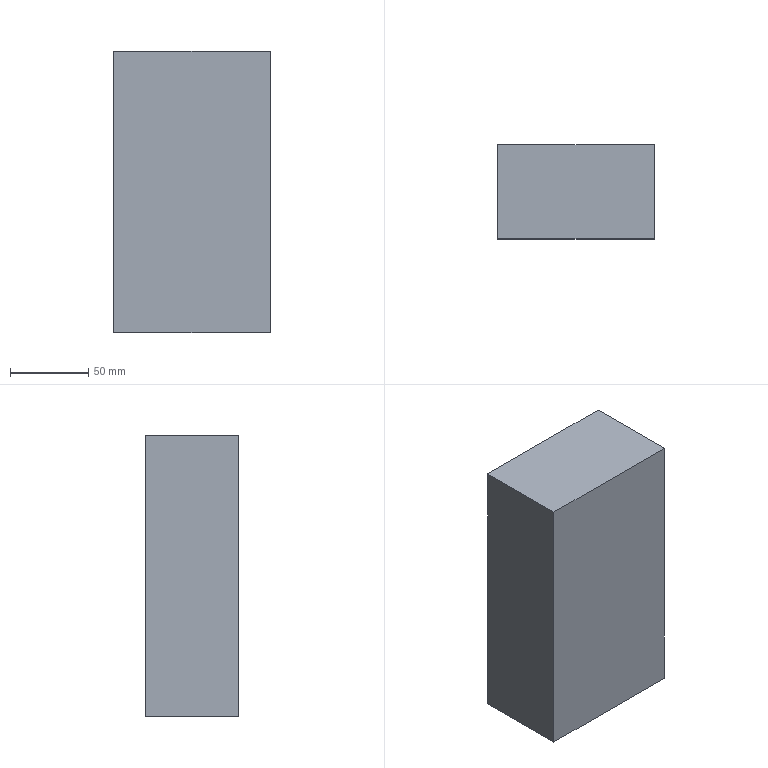Part | NX | features 28 2 | 1 solid | 10 faces | box 100 x 60 x 180 mm | volume 1074073 mm3 | plane 6 | cylinder 2 | cone 2 | commonest cylinder face diameters 10.3 x2
STEP:
#1=CARTESIAN_POINT('',(2254.85,742.5,-113.));
#2=VERTEX_POINT('',#1);
#3=CARTESIAN_POINT('',(2260.,742.5,-113.));
#4=DIRECTION('',(0.,0.,-1.));
#5=DIRECTION('',(-1.,0.,0.));
#6=AXIS2_PLACEMENT_3D('',#3,#4,#5);
#7=CIRCLE('',#6,5.15);
#8=EDGE_CURVE('',#2,#2,#7,.T.);
#9=ORIENTED_EDGE('',*,*,#8,.F.);
#10=EDGE_LOOP('',(#9));
#11=FACE_BOUND('',#10,.T.);
#12=CARTESIAN_POINT('',(2240.,712.5,-113.));
#13=VERTEX_POINT('',#12);
#14=CARTESIAN_POINT('',(2240.,772.5,-113.));
#15=VERTEX_POINT('',#14);
#16=CARTESIAN_POINT('',(2240.,387.5,-113.));
#17=DIRECTION('',(0.,1.,0.));
#18=VECTOR('',#17,1000.);
#19=LINE('',#16,#18);
#20=EDGE_CURVE('',#13,#15,#19,.T.);
#21=ORIENTED_EDGE('',*,*,#20,.T.);
#22=CARTESIAN_POINT('',(2340.,772.5,-113.));
#23=VERTEX_POINT('',#22);
#24=CARTESIAN_POINT('',(3179.121,772.5,-113.));
#25=DIRECTION('',(1.,0.,0.));
#26=VECTOR('',#25,1000.);
#27=LINE('',#24,#26);
#28=EDGE_CURVE('',#15,#23,#27,.T.);
#29=ORIENTED_EDGE('',*,*,#28,.T.);
#30=CARTESIAN_POINT('',(2340.,712.5,-113.));
#31=VERTEX_POINT('',#30);
#32=CARTESIAN_POINT('',(2340.,772.5,-113.));
#33=DIRECTION('',(0.,1.,0.));
#34=VECTOR('',#33,1000.);
#35=LINE('',#32,#34);
#36=EDGE_CURVE('',#31,#23,#35,.T.);
#37=ORIENTED_EDGE('',*,*,#36,.F.);
#38=CARTESIAN_POINT('',(3179.121,712.5,-113.));
#39=DIRECTION('',(-1.,0.,0.));
#40=VECTOR('',#39,1000.);
#41=LINE('',#38,#40);
#42=EDGE_CURVE('',#31,#13,#41,.T.);
#43=ORIENTED_EDGE('',*,*,#42,.T.);
#44=EDGE_LOOP('',(#21,#29,#37,#43));
#45=FACE_BOUND('',#44,.T.);
#46=CARTESIAN_POINT('',(2314.85,742.5,-113.));
#47=VERTEX_POINT('',#46);
#48=CARTESIAN_POINT('',(2320.,742.5,-113.));
#49=DIRECTION('',(0.,0.,-1.));
#50=DIRECTION('',(-1.,0.,0.));
#51=AXIS2_PLACEMENT_3D('',#48,#49,#50);
#52=CIRCLE('',#51,5.15);
#53=EDGE_CURVE('',#47,#47,#52,.T.);
#54=ORIENTED_EDGE('',*,*,#53,.F.);
#55=EDGE_LOOP('',(#54));
#56=FACE_BOUND('',#55,.T.);
#57=CARTESIAN_POINT('',(3179.121,387.5,-113.));
#58=DIRECTION('',(0.,0.,-1.));
#59=DIRECTION('',(1.,0.,0.));
#60=AXIS2_PLACEMENT_3D('',#57,#58,#59);
#61=PLANE('',#60);
#62=ADVANCED_FACE('',(#11,#45,#56),#61,.T.);
#63=CARTESIAN_POINT('',(2340.,712.5,67.));
#64=VERTEX_POINT('',#63);
#65=CARTESIAN_POINT('',(2240.,712.5,67.));
#66=VERTEX_POINT('',#65);
#67=CARTESIAN_POINT('',(4085.,712.5,67.));
#68=DIRECTION('',(-1.,0.,0.));
#69=VECTOR('',#68,1000.);
#70=LINE('',#67,#69);
#71=EDGE_CURVE('',#64,#66,#70,.T.);
#72=ORIENTED_EDGE('',*,*,#71,.F.);
#73=CARTESIAN_POINT('',(2340.,772.5,67.));
#74=VERTEX_POINT('',#73);
#75=CARTESIAN_POINT('',(2340.,572.5,67.));
#76=DIRECTION('',(0.,-1.,0.));
#77=VECTOR('',#76,1000.);
#78=LINE('',#75,#77);
#79=EDGE_CURVE('',#74,#64,#78,.T.);
#80=ORIENTED_EDGE('',*,*,#79,.F.);
#81=CARTESIAN_POINT('',(2240.,772.5,67.));
#82=VERTEX_POINT('',#81);
#83=CARTESIAN_POINT('',(4085.,772.5,67.));
#84=DIRECTION('',(1.,0.,0.));
#85=VECTOR('',#84,1000.);
#86=LINE('',#83,#85);
#87=EDGE_CURVE('',#82,#74,#86,.T.);
#88=ORIENTED_EDGE('',*,*,#87,.F.);
#89=CARTESIAN_POINT('',(2240.,572.5,67.));
#90=DIRECTION('',(0.,1.,0.));
#91=VECTOR('',#90,1000.);
#92=LINE('',#89,#91);
#93=EDGE_CURVE('',#66,#82,#92,.T.);
#94=ORIENTED_EDGE('',*,*,#93,.F.);
#95=EDGE_LOOP('',(#72,#80,#88,#94));
#96=FACE_BOUND('',#95,.T.);
#97=CARTESIAN_POINT('',(4085.,572.5,67.));
#98=DIRECTION('',(0.,0.,1.));
#99=DIRECTION('',(0.,1.,0.));
#100=AXIS2_PLACEMENT_3D('',#97,#98,#99);
#101=PLANE('',#100);
#102=ADVANCED_FACE('',(#96),#101,.T.);
#103=CARTESIAN_POINT('',(2340.,712.5,-113.));
#104=DIRECTION('',(0.,0.,-1.));
#105=VECTOR('',#104,1000.);
#106=LINE('',#103,#105);
#107=EDGE_CURVE('',#64,#31,#106,.T.);
#108=ORIENTED_EDGE('',*,*,#107,.T.);
#109=ORIENTED_EDGE('',*,*,#36,.T.);
#110=CARTESIAN_POINT('',(2340.,772.5,-113.));
#111=DIRECTION('',(0.,0.,1.));
#112=VECTOR('',#111,1000.);
#113=LINE('',#110,#112);
#114=EDGE_CURVE('',#23,#74,#113,.T.);
#115=ORIENTED_EDGE('',*,*,#114,.T.);
#116=ORIENTED_EDGE('',*,*,#79,.T.);
#117=EDGE_LOOP('',(#108,#109,#115,#116));
#118=FACE_BOUND('',#117,.T.);
#119=CARTESIAN_POINT('',(2340.,772.5,-113.));
#120=DIRECTION('',(1.,0.,0.));
#121=DIRECTION('',(0.,0.,1.));
#122=AXIS2_PLACEMENT_3D('',#119,#120,#121);
#123=PLANE('',#122);
#124=ADVANCED_FACE('',(#118),#123,.T.);
#125=ORIENTED_EDGE('',*,*,#114,.F.);
#126=ORIENTED_EDGE('',*,*,#28,.F.);
#127=CARTESIAN_POINT('',(2240.,772.5,-113.));
#128=DIRECTION('',(0.,0.,-1.));
#129=VECTOR('',#128,1000.);
#130=LINE('',#127,#129);
#131=EDGE_CURVE('',#82,#15,#130,.T.);
#132=ORIENTED_EDGE('',*,*,#131,.F.);
#133=ORIENTED_EDGE('',*,*,#87,.T.);
#134=EDGE_LOOP('',(#125,#126,#132,#133));
#135=FACE_BOUND('',#134,.T.);
#136=CARTESIAN_POINT('',(2270.,772.5,-113.));
#137=DIRECTION('',(0.,1.,0.));
#138=DIRECTION('',(0.,0.,1.));
#139=AXIS2_PLACEMENT_3D('',#136,#137,#138);
#140=PLANE('',#139);
#141=ADVANCED_FACE('',(#135),#140,.T.);
#142=ORIENTED_EDGE('',*,*,#131,.T.);
#143=ORIENTED_EDGE('',*,*,#20,.F.);
#144=CARTESIAN_POINT('',(2240.,712.5,-113.));
#145=DIRECTION('',(0.,0.,1.));
#146=VECTOR('',#145,1000.);
#147=LINE('',#144,#146);
#148=EDGE_CURVE('',#13,#66,#147,.T.);
#149=ORIENTED_EDGE('',*,*,#148,.T.);
#150=ORIENTED_EDGE('',*,*,#93,.T.);
#151=EDGE_LOOP('',(#142,#143,#149,#150));
#152=FACE_BOUND('',#151,.T.);
#153=CARTESIAN_POINT('',(2240.,772.5,-113.));
#154=DIRECTION('',(-1.,0.,0.));
#155=DIRECTION('',(0.,0.,-1.));
#156=AXIS2_PLACEMENT_3D('',#153,#154,#155);
#157=PLANE('',#156);
#158=ADVANCED_FACE('',(#152),#157,.T.);
#159=ORIENTED_EDGE('',*,*,#148,.F.);
#160=ORIENTED_EDGE('',*,*,#42,.F.);
#161=ORIENTED_EDGE('',*,*,#107,.F.);
#162=ORIENTED_EDGE('',*,*,#71,.T.);
#163=EDGE_LOOP('',(#159,#160,#161,#162));
#164=FACE_BOUND('',#163,.T.);
#165=CARTESIAN_POINT('',(2270.,712.5,-113.));
#166=DIRECTION('',(0.,-1.,0.));
#167=DIRECTION('',(0.,0.,-1.));
#168=AXIS2_PLACEMENT_3D('',#165,#166,#167);
#169=PLANE('',#168);
#170=ADVANCED_FACE('',(#164),#169,.T.);
#171=CARTESIAN_POINT('',(2254.85,742.5,-79.15));
#172=VERTEX_POINT('',#171);
#173=CARTESIAN_POINT('',(2260.,742.5,-79.15));
#174=DIRECTION('',(0.,0.,-1.));
#175=DIRECTION('',(-1.,0.,0.));
#176=AXIS2_PLACEMENT_3D('',#173,#174,#175);
#177=CIRCLE('',#176,5.15);
#178=EDGE_CURVE('',#172,#172,#177,.T.);
#179=ORIENTED_EDGE('',*,*,#178,.F.);
#180=EDGE_LOOP('',(#179));
#181=FACE_BOUND('',#180,.T.);
#182=ORIENTED_EDGE('',*,*,#8,.T.);
#183=EDGE_LOOP('',(#182));
#184=FACE_BOUND('',#183,.T.);
#185=CARTESIAN_POINT('',(2260.,742.5,-113.));
#186=DIRECTION('',(0.,0.,1.));
#187=DIRECTION('',(0.,1.,0.));
#188=AXIS2_PLACEMENT_3D('',#185,#186,#187);
#189=CYLINDRICAL_SURFACE('',#188,5.15);
#190=ADVANCED_FACE('',(#181,#184),#189,.F.);
#191=CARTESIAN_POINT('',(2260.,742.5,-74.));
#192=VERTEX_POINT('',#191);
#193=VERTEX_LOOP('',#192);
#194=FACE_BOUND('',#193,.T.);
#195=ORIENTED_EDGE('',*,*,#178,.T.);
#196=EDGE_LOOP('',(#195));
#197=FACE_BOUND('',#196,.T.);
#198=CARTESIAN_POINT('',(2260.,742.5,-79.149));
#199=DIRECTION('',(0.,0.,-1.));
#200=DIRECTION('',(0.,-1.,0.));
#201=AXIS2_PLACEMENT_3D('',#198,#199,#200);
#202=CONICAL_SURFACE('',#201,5.149,0.7854);
#203=ADVANCED_FACE('',(#194,#197),#202,.F.);
#204=CARTESIAN_POINT('',(2314.85,742.5,-79.15));
#205=VERTEX_POINT('',#204);
#206=CARTESIAN_POINT('',(2320.,742.5,-79.15));
#207=DIRECTION('',(0.,0.,-1.));
#208=DIRECTION('',(-1.,0.,0.));
#209=AXIS2_PLACEMENT_3D('',#206,#207,#208);
#210=CIRCLE('',#209,5.15);
#211=EDGE_CURVE('',#205,#205,#210,.T.);
#212=ORIENTED_EDGE('',*,*,#211,.F.);
#213=EDGE_LOOP('',(#212));
#214=FACE_BOUND('',#213,.T.);
#215=ORIENTED_EDGE('',*,*,#53,.T.);
#216=EDGE_LOOP('',(#215));
#217=FACE_BOUND('',#216,.T.);
#218=CARTESIAN_POINT('',(2320.,742.5,-113.));
#219=DIRECTION('',(0.,0.,1.));
#220=DIRECTION('',(0.,1.,0.));
#221=AXIS2_PLACEMENT_3D('',#218,#219,#220);
#222=CYLINDRICAL_SURFACE('',#221,5.15);
#223=ADVANCED_FACE('',(#214,#217),#222,.F.);
#224=CARTESIAN_POINT('',(2320.,742.5,-74.));
#225=VERTEX_POINT('',#224);
#226=VERTEX_LOOP('',#225);
#227=FACE_BOUND('',#226,.T.);
#228=ORIENTED_EDGE('',*,*,#211,.T.);
#229=EDGE_LOOP('',(#228));
#230=FACE_BOUND('',#229,.T.);
#231=CARTESIAN_POINT('',(2320.,742.5,-79.149));
#232=DIRECTION('',(0.,0.,-1.));
#233=DIRECTION('',(0.,-1.,0.));
#234=AXIS2_PLACEMENT_3D('',#231,#232,#233);
#235=CONICAL_SURFACE('',#234,5.149,0.7854);
#236=ADVANCED_FACE('',(#227,#230),#235,.F.);
#237=CLOSED_SHELL('',(#62,#102,#124,#141,#158,#170,#190,#203,#223,#236));
#238=MANIFOLD_SOLID_BREP('',#237);
#239=(LENGTH_UNIT()NAMED_UNIT(*)SI_UNIT(.MILLI.,.METRE.));
#240=UNCERTAINTY_MEASURE_WITH_UNIT(LENGTH_MEASURE(0.00001),#239,'','');
#241=(NAMED_UNIT(*)PLANE_ANGLE_UNIT()SI_UNIT($,.RADIAN.));
#242=(NAMED_UNIT(*)SI_UNIT($,.STERADIAN.)SOLID_ANGLE_UNIT());
#243=(GEOMETRIC_REPRESENTATION_CONTEXT(3)GLOBAL_UNCERTAINTY_ASSIGNED_CONTEXT((#240))GLOBAL_UNIT_ASSIGNED_CONTEXT((#239,#241,#242))REPRESENTATION_CONTEXT('',''));
#244=ADVANCED_BREP_SHAPE_REPRESENTATION('',(#238),#243);